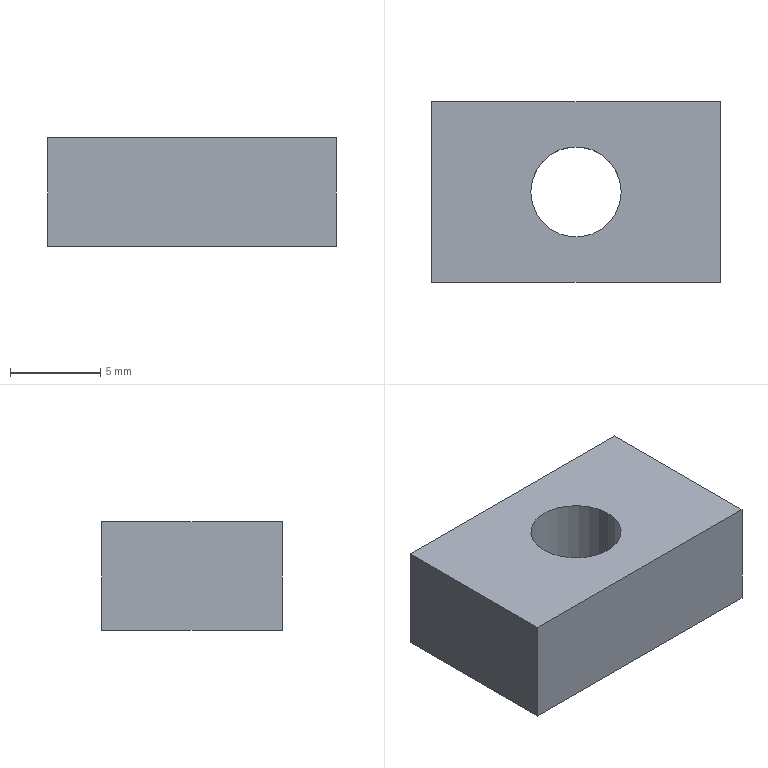Part | SolidWorks | features Extrusion 1, HoleWzd 1 | 1 solid | 8 faces | box 16 x 10 x 6 mm | volume 842.19 mm3 | plane 6 | cylinder 2 | commonest cylinder face diameters 5 x2
STEP:
#1=CARTESIAN_POINT('',(-2.5,0.,0.));
#2=VERTEX_POINT('',#1);
#3=CARTESIAN_POINT('',(2.5,0.,0.));
#4=VERTEX_POINT('',#3);
#5=CARTESIAN_POINT('',(0.,0.,0.));
#6=DIRECTION('',(0.,0.,1.));
#7=DIRECTION('',(1.,0.,0.));
#8=AXIS2_PLACEMENT_3D('',#5,#6,#7);
#9=CIRCLE('',#8,2.5);
#10=EDGE_CURVE('',#2,#4,#9,.T.);
#11=ORIENTED_EDGE('',*,*,#10,.F.);
#12=CARTESIAN_POINT('',(-2.5,0.,6.));
#13=VERTEX_POINT('',#12);
#14=CARTESIAN_POINT('',(-2.5,0.,6.));
#15=DIRECTION('',(0.,0.,1.));
#16=VECTOR('',#15,1000.);
#17=LINE('',#14,#16);
#18=EDGE_CURVE('',#2,#13,#17,.T.);
#19=ORIENTED_EDGE('',*,*,#18,.T.);
#20=CARTESIAN_POINT('',(2.5,0.,6.));
#21=VERTEX_POINT('',#20);
#22=CARTESIAN_POINT('',(0.,0.,6.));
#23=DIRECTION('',(0.,0.,1.));
#24=DIRECTION('',(1.,0.,0.));
#25=AXIS2_PLACEMENT_3D('',#22,#23,#24);
#26=CIRCLE('',#25,2.5);
#27=EDGE_CURVE('',#13,#21,#26,.T.);
#28=ORIENTED_EDGE('',*,*,#27,.T.);
#29=CARTESIAN_POINT('',(2.5,0.,6.));
#30=DIRECTION('',(0.,0.,1.));
#31=VECTOR('',#30,1000.);
#32=LINE('',#29,#31);
#33=EDGE_CURVE('',#4,#21,#32,.T.);
#34=ORIENTED_EDGE('',*,*,#33,.F.);
#35=EDGE_LOOP('',(#11,#19,#28,#34));
#36=FACE_OUTER_BOUND('',#35,.T.);
#37=CARTESIAN_POINT('',(0.,0.,6.));
#38=DIRECTION('',(0.,0.,1.));
#39=DIRECTION('',(1.,0.,0.));
#40=AXIS2_PLACEMENT_3D('',#37,#38,#39);
#41=CYLINDRICAL_SURFACE('',#40,2.5);
#42=ADVANCED_FACE('',(#36),#41,.F.);
#43=CARTESIAN_POINT('',(-8.,5.,0.));
#44=VERTEX_POINT('',#43);
#45=CARTESIAN_POINT('',(-8.,-5.,0.));
#46=VERTEX_POINT('',#45);
#47=CARTESIAN_POINT('',(-8.,-5.,0.));
#48=DIRECTION('',(0.,-1.,0.));
#49=VECTOR('',#48,1000.);
#50=LINE('',#47,#49);
#51=EDGE_CURVE('',#44,#46,#50,.T.);
#52=ORIENTED_EDGE('',*,*,#51,.T.);
#53=CARTESIAN_POINT('',(-8.,-5.,6.));
#54=VERTEX_POINT('',#53);
#55=CARTESIAN_POINT('',(-8.,-5.,6.));
#56=DIRECTION('',(0.,0.,-1.));
#57=VECTOR('',#56,1000.);
#58=LINE('',#55,#57);
#59=EDGE_CURVE('',#54,#46,#58,.T.);
#60=ORIENTED_EDGE('',*,*,#59,.F.);
#61=CARTESIAN_POINT('',(-8.,5.,6.));
#62=VERTEX_POINT('',#61);
#63=CARTESIAN_POINT('',(-8.,-5.,6.));
#64=DIRECTION('',(0.,-1.,0.));
#65=VECTOR('',#64,1000.);
#66=LINE('',#63,#65);
#67=EDGE_CURVE('',#62,#54,#66,.T.);
#68=ORIENTED_EDGE('',*,*,#67,.F.);
#69=CARTESIAN_POINT('',(-8.,5.,6.));
#70=DIRECTION('',(0.,0.,-1.));
#71=VECTOR('',#70,1000.);
#72=LINE('',#69,#71);
#73=EDGE_CURVE('',#62,#44,#72,.T.);
#74=ORIENTED_EDGE('',*,*,#73,.T.);
#75=EDGE_LOOP('',(#52,#60,#68,#74));
#76=FACE_OUTER_BOUND('',#75,.T.);
#77=CARTESIAN_POINT('',(-8.,-5.,6.));
#78=DIRECTION('',(1.,0.,0.));
#79=DIRECTION('',(0.,0.,-1.));
#80=AXIS2_PLACEMENT_3D('',#77,#78,#79);
#81=PLANE('',#80);
#82=ADVANCED_FACE('',(#76),#81,.F.);
#83=CARTESIAN_POINT('',(8.,-5.,0.));
#84=VERTEX_POINT('',#83);
#85=CARTESIAN_POINT('',(8.,-5.,0.));
#86=DIRECTION('',(1.,0.,0.));
#87=VECTOR('',#86,1000.);
#88=LINE('',#85,#87);
#89=EDGE_CURVE('',#46,#84,#88,.T.);
#90=ORIENTED_EDGE('',*,*,#89,.T.);
#91=CARTESIAN_POINT('',(8.,-5.,6.));
#92=VERTEX_POINT('',#91);
#93=CARTESIAN_POINT('',(8.,-5.,6.));
#94=DIRECTION('',(0.,0.,-1.));
#95=VECTOR('',#94,1000.);
#96=LINE('',#93,#95);
#97=EDGE_CURVE('',#92,#84,#96,.T.);
#98=ORIENTED_EDGE('',*,*,#97,.F.);
#99=CARTESIAN_POINT('',(8.,-5.,6.));
#100=DIRECTION('',(1.,0.,0.));
#101=VECTOR('',#100,1000.);
#102=LINE('',#99,#101);
#103=EDGE_CURVE('',#54,#92,#102,.T.);
#104=ORIENTED_EDGE('',*,*,#103,.F.);
#105=ORIENTED_EDGE('',*,*,#59,.T.);
#106=EDGE_LOOP('',(#90,#98,#104,#105));
#107=FACE_OUTER_BOUND('',#106,.T.);
#108=CARTESIAN_POINT('',(8.,-5.,6.));
#109=DIRECTION('',(0.,1.,0.));
#110=DIRECTION('',(-1.,0.,0.));
#111=AXIS2_PLACEMENT_3D('',#108,#109,#110);
#112=PLANE('',#111);
#113=ADVANCED_FACE('',(#107),#112,.F.);
#114=CARTESIAN_POINT('',(8.,5.,0.));
#115=VERTEX_POINT('',#114);
#116=CARTESIAN_POINT('',(8.,-5.,0.));
#117=DIRECTION('',(0.,1.,0.));
#118=VECTOR('',#117,1000.);
#119=LINE('',#116,#118);
#120=EDGE_CURVE('',#84,#115,#119,.T.);
#121=ORIENTED_EDGE('',*,*,#120,.T.);
#122=CARTESIAN_POINT('',(8.,5.,6.));
#123=VERTEX_POINT('',#122);
#124=CARTESIAN_POINT('',(8.,5.,6.));
#125=DIRECTION('',(0.,0.,-1.));
#126=VECTOR('',#125,1000.);
#127=LINE('',#124,#126);
#128=EDGE_CURVE('',#123,#115,#127,.T.);
#129=ORIENTED_EDGE('',*,*,#128,.F.);
#130=CARTESIAN_POINT('',(8.,-5.,6.));
#131=DIRECTION('',(0.,1.,0.));
#132=VECTOR('',#131,1000.);
#133=LINE('',#130,#132);
#134=EDGE_CURVE('',#92,#123,#133,.T.);
#135=ORIENTED_EDGE('',*,*,#134,.F.);
#136=ORIENTED_EDGE('',*,*,#97,.T.);
#137=EDGE_LOOP('',(#121,#129,#135,#136));
#138=FACE_OUTER_BOUND('',#137,.T.);
#139=CARTESIAN_POINT('',(8.,-5.,6.));
#140=DIRECTION('',(-1.,0.,0.));
#141=DIRECTION('',(0.,0.,1.));
#142=AXIS2_PLACEMENT_3D('',#139,#140,#141);
#143=PLANE('',#142);
#144=ADVANCED_FACE('',(#138),#143,.F.);
#145=CARTESIAN_POINT('',(8.,5.,0.));
#146=DIRECTION('',(-1.,0.,0.));
#147=VECTOR('',#146,1000.);
#148=LINE('',#145,#147);
#149=EDGE_CURVE('',#115,#44,#148,.T.);
#150=ORIENTED_EDGE('',*,*,#149,.T.);
#151=ORIENTED_EDGE('',*,*,#73,.F.);
#152=CARTESIAN_POINT('',(8.,5.,6.));
#153=DIRECTION('',(-1.,0.,0.));
#154=VECTOR('',#153,1000.);
#155=LINE('',#152,#154);
#156=EDGE_CURVE('',#123,#62,#155,.T.);
#157=ORIENTED_EDGE('',*,*,#156,.F.);
#158=ORIENTED_EDGE('',*,*,#128,.T.);
#159=EDGE_LOOP('',(#150,#151,#157,#158));
#160=FACE_OUTER_BOUND('',#159,.T.);
#161=CARTESIAN_POINT('',(8.,5.,6.));
#162=DIRECTION('',(0.,-1.,0.));
#163=DIRECTION('',(1.,0.,0.));
#164=AXIS2_PLACEMENT_3D('',#161,#162,#163);
#165=PLANE('',#164);
#166=ADVANCED_FACE('',(#160),#165,.F.);
#167=CARTESIAN_POINT('',(0.,0.,6.));
#168=DIRECTION('',(0.,0.,1.));
#169=DIRECTION('',(1.,0.,0.));
#170=AXIS2_PLACEMENT_3D('',#167,#168,#169);
#171=CIRCLE('',#170,2.5);
#172=EDGE_CURVE('',#21,#13,#171,.T.);
#173=ORIENTED_EDGE('',*,*,#172,.F.);
#174=ORIENTED_EDGE('',*,*,#27,.F.);
#175=EDGE_LOOP('',(#173,#174));
#176=FACE_BOUND('',#175,.T.);
#177=ORIENTED_EDGE('',*,*,#67,.T.);
#178=ORIENTED_EDGE('',*,*,#103,.T.);
#179=ORIENTED_EDGE('',*,*,#134,.T.);
#180=ORIENTED_EDGE('',*,*,#156,.T.);
#181=EDGE_LOOP('',(#177,#178,#179,#180));
#182=FACE_OUTER_BOUND('',#181,.T.);
#183=CARTESIAN_POINT('',(0.,0.,6.));
#184=DIRECTION('',(0.,0.,1.));
#185=DIRECTION('',(1.,0.,0.));
#186=AXIS2_PLACEMENT_3D('',#183,#184,#185);
#187=PLANE('',#186);
#188=ADVANCED_FACE('',(#176,#182),#187,.T.);
#189=CARTESIAN_POINT('',(0.,0.,0.));
#190=DIRECTION('',(0.,0.,1.));
#191=DIRECTION('',(1.,0.,0.));
#192=AXIS2_PLACEMENT_3D('',#189,#190,#191);
#193=CIRCLE('',#192,2.5);
#194=EDGE_CURVE('',#4,#2,#193,.T.);
#195=ORIENTED_EDGE('',*,*,#194,.T.);
#196=ORIENTED_EDGE('',*,*,#10,.T.);
#197=EDGE_LOOP('',(#195,#196));
#198=FACE_BOUND('',#197,.T.);
#199=ORIENTED_EDGE('',*,*,#51,.F.);
#200=ORIENTED_EDGE('',*,*,#149,.F.);
#201=ORIENTED_EDGE('',*,*,#120,.F.);
#202=ORIENTED_EDGE('',*,*,#89,.F.);
#203=EDGE_LOOP('',(#199,#200,#201,#202));
#204=FACE_OUTER_BOUND('',#203,.T.);
#205=CARTESIAN_POINT('',(0.,0.,0.));
#206=DIRECTION('',(0.,0.,1.));
#207=DIRECTION('',(1.,0.,0.));
#208=AXIS2_PLACEMENT_3D('',#205,#206,#207);
#209=PLANE('',#208);
#210=ADVANCED_FACE('',(#198,#204),#209,.F.);
#211=ORIENTED_EDGE('',*,*,#18,.F.);
#212=ORIENTED_EDGE('',*,*,#194,.F.);
#213=ORIENTED_EDGE('',*,*,#33,.T.);
#214=ORIENTED_EDGE('',*,*,#172,.T.);
#215=EDGE_LOOP('',(#211,#212,#213,#214));
#216=FACE_OUTER_BOUND('',#215,.T.);
#217=CARTESIAN_POINT('',(0.,0.,6.));
#218=DIRECTION('',(0.,0.,1.));
#219=DIRECTION('',(1.,0.,0.));
#220=AXIS2_PLACEMENT_3D('',#217,#218,#219);
#221=CYLINDRICAL_SURFACE('',#220,2.5);
#222=ADVANCED_FACE('',(#216),#221,.F.);
#223=CLOSED_SHELL('',(#42,#82,#113,#144,#166,#188,#210,#222));
#224=MANIFOLD_SOLID_BREP('',#223);
#225=CARTESIAN_POINT('',(0.,0.,0.));
#226=DIRECTION('',(0.,0.,1.));
#227=DIRECTION('',(1.,0.,0.));
#228=AXIS2_PLACEMENT_3D('',#225,#226,#227);
#229=(LENGTH_UNIT()NAMED_UNIT(*)SI_UNIT(.MILLI.,.METRE.));
#230=UNCERTAINTY_MEASURE_WITH_UNIT(LENGTH_MEASURE(0.00001),#229,'','');
#231=(NAMED_UNIT(*)PLANE_ANGLE_UNIT()SI_UNIT($,.RADIAN.));
#232=(NAMED_UNIT(*)SI_UNIT($,.STERADIAN.)SOLID_ANGLE_UNIT());
#233=(GEOMETRIC_REPRESENTATION_CONTEXT(3)GLOBAL_UNCERTAINTY_ASSIGNED_CONTEXT((#230))GLOBAL_UNIT_ASSIGNED_CONTEXT((#229,#231,#232))REPRESENTATION_CONTEXT('',''));
#234=ADVANCED_BREP_SHAPE_REPRESENTATION('',(#224,#228),#233);